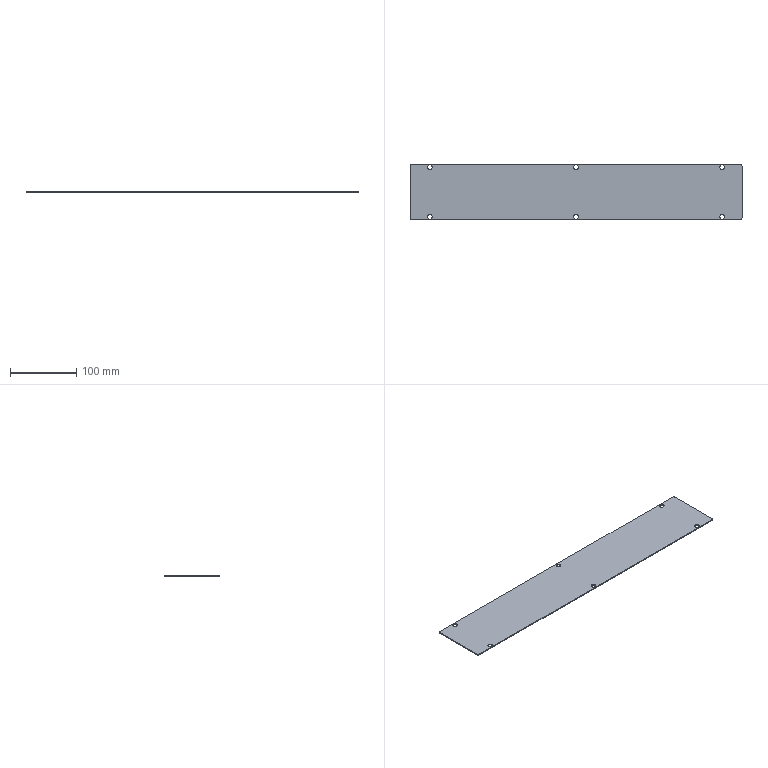Part | SolidWorks | features Cut 1, Extrusion 1, Fillet 1 | 1 solid | 22 faces | box 500 x 84 x 1.5 mm | volume 62642 mm3 | cylinder 16 | plane 6 | commonest cylinder face diameters 7 x12 6 x4
STEP:
#1=CARTESIAN_POINT('',(223.5,37.5,1.5));
#2=VERTEX_POINT('',#1);
#3=CARTESIAN_POINT('',(216.5,37.5,1.5));
#4=VERTEX_POINT('',#3);
#5=CARTESIAN_POINT('',(220.,37.5,1.5));
#6=DIRECTION('',(0.,0.,-1.));
#7=DIRECTION('',(1.,0.,0.));
#8=AXIS2_PLACEMENT_3D('',#5,#6,#7);
#9=CIRCLE('',#8,3.5);
#10=EDGE_CURVE('',#2,#4,#9,.T.);
#11=ORIENTED_EDGE('',*,*,#10,.F.);
#12=CARTESIAN_POINT('',(223.5,37.5,0.));
#13=VERTEX_POINT('',#12);
#14=CARTESIAN_POINT('',(223.5,37.5,1.5));
#15=DIRECTION('',(0.,0.,-1.));
#16=VECTOR('',#15,1000.);
#17=LINE('',#14,#16);
#18=EDGE_CURVE('',#2,#13,#17,.T.);
#19=ORIENTED_EDGE('',*,*,#18,.T.);
#20=CARTESIAN_POINT('',(216.5,37.5,0.));
#21=VERTEX_POINT('',#20);
#22=CARTESIAN_POINT('',(220.,37.5,0.));
#23=DIRECTION('',(0.,0.,-1.));
#24=DIRECTION('',(1.,0.,0.));
#25=AXIS2_PLACEMENT_3D('',#22,#23,#24);
#26=CIRCLE('',#25,3.5);
#27=EDGE_CURVE('',#13,#21,#26,.T.);
#28=ORIENTED_EDGE('',*,*,#27,.T.);
#29=CARTESIAN_POINT('',(216.5,37.5,1.5));
#30=DIRECTION('',(0.,0.,-1.));
#31=VECTOR('',#30,1000.);
#32=LINE('',#29,#31);
#33=EDGE_CURVE('',#4,#21,#32,.T.);
#34=ORIENTED_EDGE('',*,*,#33,.F.);
#35=EDGE_LOOP('',(#11,#19,#28,#34));
#36=FACE_OUTER_BOUND('',#35,.T.);
#37=CARTESIAN_POINT('',(220.,37.5,1.5));
#38=DIRECTION('',(0.,0.,-1.));
#39=DIRECTION('',(-1.,0.,0.));
#40=AXIS2_PLACEMENT_3D('',#37,#38,#39);
#41=CYLINDRICAL_SURFACE('',#40,3.5);
#42=ADVANCED_FACE('',(#36),#41,.F.);
#43=CARTESIAN_POINT('',(-216.5,37.5,1.5));
#44=VERTEX_POINT('',#43);
#45=CARTESIAN_POINT('',(-223.5,37.5,1.5));
#46=VERTEX_POINT('',#45);
#47=CARTESIAN_POINT('',(-220.,37.5,1.5));
#48=DIRECTION('',(0.,0.,-1.));
#49=DIRECTION('',(1.,0.,0.));
#50=AXIS2_PLACEMENT_3D('',#47,#48,#49);
#51=CIRCLE('',#50,3.5);
#52=EDGE_CURVE('',#44,#46,#51,.T.);
#53=ORIENTED_EDGE('',*,*,#52,.F.);
#54=CARTESIAN_POINT('',(-216.5,37.5,0.));
#55=VERTEX_POINT('',#54);
#56=CARTESIAN_POINT('',(-216.5,37.5,1.5));
#57=DIRECTION('',(0.,0.,-1.));
#58=VECTOR('',#57,1000.);
#59=LINE('',#56,#58);
#60=EDGE_CURVE('',#44,#55,#59,.T.);
#61=ORIENTED_EDGE('',*,*,#60,.T.);
#62=CARTESIAN_POINT('',(-223.5,37.5,0.));
#63=VERTEX_POINT('',#62);
#64=CARTESIAN_POINT('',(-220.,37.5,0.));
#65=DIRECTION('',(0.,0.,-1.));
#66=DIRECTION('',(1.,0.,0.));
#67=AXIS2_PLACEMENT_3D('',#64,#65,#66);
#68=CIRCLE('',#67,3.5);
#69=EDGE_CURVE('',#55,#63,#68,.T.);
#70=ORIENTED_EDGE('',*,*,#69,.T.);
#71=CARTESIAN_POINT('',(-223.5,37.5,1.5));
#72=DIRECTION('',(0.,0.,-1.));
#73=VECTOR('',#72,1000.);
#74=LINE('',#71,#73);
#75=EDGE_CURVE('',#46,#63,#74,.T.);
#76=ORIENTED_EDGE('',*,*,#75,.F.);
#77=EDGE_LOOP('',(#53,#61,#70,#76));
#78=FACE_OUTER_BOUND('',#77,.T.);
#79=CARTESIAN_POINT('',(-220.,37.5,1.5));
#80=DIRECTION('',(0.,0.,-1.));
#81=DIRECTION('',(-1.,0.,0.));
#82=AXIS2_PLACEMENT_3D('',#79,#80,#81);
#83=CYLINDRICAL_SURFACE('',#82,3.5);
#84=ADVANCED_FACE('',(#78),#83,.F.);
#85=CARTESIAN_POINT('',(3.5,-37.5,1.5));
#86=VERTEX_POINT('',#85);
#87=CARTESIAN_POINT('',(-3.5,-37.5,1.5));
#88=VERTEX_POINT('',#87);
#89=CARTESIAN_POINT('',(0.,-37.5,1.5));
#90=DIRECTION('',(0.,0.,-1.));
#91=DIRECTION('',(-1.,0.,0.));
#92=AXIS2_PLACEMENT_3D('',#89,#90,#91);
#93=CIRCLE('',#92,3.5);
#94=EDGE_CURVE('',#86,#88,#93,.T.);
#95=ORIENTED_EDGE('',*,*,#94,.F.);
#96=CARTESIAN_POINT('',(3.5,-37.5,0.));
#97=VERTEX_POINT('',#96);
#98=CARTESIAN_POINT('',(3.5,-37.5,1.5));
#99=DIRECTION('',(0.,0.,-1.));
#100=VECTOR('',#99,1000.);
#101=LINE('',#98,#100);
#102=EDGE_CURVE('',#86,#97,#101,.T.);
#103=ORIENTED_EDGE('',*,*,#102,.T.);
#104=CARTESIAN_POINT('',(-3.5,-37.5,0.));
#105=VERTEX_POINT('',#104);
#106=CARTESIAN_POINT('',(0.,-37.5,0.));
#107=DIRECTION('',(0.,0.,-1.));
#108=DIRECTION('',(-1.,0.,0.));
#109=AXIS2_PLACEMENT_3D('',#106,#107,#108);
#110=CIRCLE('',#109,3.5);
#111=EDGE_CURVE('',#97,#105,#110,.T.);
#112=ORIENTED_EDGE('',*,*,#111,.T.);
#113=CARTESIAN_POINT('',(-3.5,-37.5,1.5));
#114=DIRECTION('',(0.,0.,-1.));
#115=VECTOR('',#114,1000.);
#116=LINE('',#113,#115);
#117=EDGE_CURVE('',#88,#105,#116,.T.);
#118=ORIENTED_EDGE('',*,*,#117,.F.);
#119=EDGE_LOOP('',(#95,#103,#112,#118));
#120=FACE_OUTER_BOUND('',#119,.T.);
#121=CARTESIAN_POINT('',(0.,-37.5,1.5));
#122=DIRECTION('',(0.,0.,-1.));
#123=DIRECTION('',(-1.,0.,0.));
#124=AXIS2_PLACEMENT_3D('',#121,#122,#123);
#125=CYLINDRICAL_SURFACE('',#124,3.5);
#126=ADVANCED_FACE('',(#120),#125,.F.);
#127=CARTESIAN_POINT('',(-216.5,-37.5,1.5));
#128=VERTEX_POINT('',#127);
#129=CARTESIAN_POINT('',(-223.5,-37.5,1.5));
#130=VERTEX_POINT('',#129);
#131=CARTESIAN_POINT('',(-220.,-37.5,1.5));
#132=DIRECTION('',(0.,0.,-1.));
#133=DIRECTION('',(-1.,0.,0.));
#134=AXIS2_PLACEMENT_3D('',#131,#132,#133);
#135=CIRCLE('',#134,3.5);
#136=EDGE_CURVE('',#128,#130,#135,.T.);
#137=ORIENTED_EDGE('',*,*,#136,.F.);
#138=CARTESIAN_POINT('',(-216.5,-37.5,0.));
#139=VERTEX_POINT('',#138);
#140=CARTESIAN_POINT('',(-216.5,-37.5,1.5));
#141=DIRECTION('',(0.,0.,-1.));
#142=VECTOR('',#141,1000.);
#143=LINE('',#140,#142);
#144=EDGE_CURVE('',#128,#139,#143,.T.);
#145=ORIENTED_EDGE('',*,*,#144,.T.);
#146=CARTESIAN_POINT('',(-223.5,-37.5,0.));
#147=VERTEX_POINT('',#146);
#148=CARTESIAN_POINT('',(-220.,-37.5,0.));
#149=DIRECTION('',(0.,0.,-1.));
#150=DIRECTION('',(-1.,0.,0.));
#151=AXIS2_PLACEMENT_3D('',#148,#149,#150);
#152=CIRCLE('',#151,3.5);
#153=EDGE_CURVE('',#139,#147,#152,.T.);
#154=ORIENTED_EDGE('',*,*,#153,.T.);
#155=CARTESIAN_POINT('',(-223.5,-37.5,1.5));
#156=DIRECTION('',(0.,0.,-1.));
#157=VECTOR('',#156,1000.);
#158=LINE('',#155,#157);
#159=EDGE_CURVE('',#130,#147,#158,.T.);
#160=ORIENTED_EDGE('',*,*,#159,.F.);
#161=EDGE_LOOP('',(#137,#145,#154,#160));
#162=FACE_OUTER_BOUND('',#161,.T.);
#163=CARTESIAN_POINT('',(-220.,-37.5,1.5));
#164=DIRECTION('',(0.,0.,-1.));
#165=DIRECTION('',(-1.,0.,0.));
#166=AXIS2_PLACEMENT_3D('',#163,#164,#165);
#167=CYLINDRICAL_SURFACE('',#166,3.5);
#168=ADVANCED_FACE('',(#162),#167,.F.);
#169=CARTESIAN_POINT('',(223.5,-37.5,1.5));
#170=VERTEX_POINT('',#169);
#171=CARTESIAN_POINT('',(216.5,-37.5,1.5));
#172=VERTEX_POINT('',#171);
#173=CARTESIAN_POINT('',(220.,-37.5,1.5));
#174=DIRECTION('',(0.,0.,-1.));
#175=DIRECTION('',(-1.,0.,0.));
#176=AXIS2_PLACEMENT_3D('',#173,#174,#175);
#177=CIRCLE('',#176,3.5);
#178=EDGE_CURVE('',#170,#172,#177,.T.);
#179=ORIENTED_EDGE('',*,*,#178,.F.);
#180=CARTESIAN_POINT('',(223.5,-37.5,0.));
#181=VERTEX_POINT('',#180);
#182=CARTESIAN_POINT('',(223.5,-37.5,1.5));
#183=DIRECTION('',(0.,0.,-1.));
#184=VECTOR('',#183,1000.);
#185=LINE('',#182,#184);
#186=EDGE_CURVE('',#170,#181,#185,.T.);
#187=ORIENTED_EDGE('',*,*,#186,.T.);
#188=CARTESIAN_POINT('',(216.5,-37.5,0.));
#189=VERTEX_POINT('',#188);
#190=CARTESIAN_POINT('',(220.,-37.5,0.));
#191=DIRECTION('',(0.,0.,-1.));
#192=DIRECTION('',(-1.,0.,0.));
#193=AXIS2_PLACEMENT_3D('',#190,#191,#192);
#194=CIRCLE('',#193,3.5);
#195=EDGE_CURVE('',#181,#189,#194,.T.);
#196=ORIENTED_EDGE('',*,*,#195,.T.);
#197=CARTESIAN_POINT('',(216.5,-37.5,1.5));
#198=DIRECTION('',(0.,0.,-1.));
#199=VECTOR('',#198,1000.);
#200=LINE('',#197,#199);
#201=EDGE_CURVE('',#172,#189,#200,.T.);
#202=ORIENTED_EDGE('',*,*,#201,.F.);
#203=EDGE_LOOP('',(#179,#187,#196,#202));
#204=FACE_OUTER_BOUND('',#203,.T.);
#205=CARTESIAN_POINT('',(220.,-37.5,1.5));
#206=DIRECTION('',(0.,0.,-1.));
#207=DIRECTION('',(-1.,0.,0.));
#208=AXIS2_PLACEMENT_3D('',#205,#206,#207);
#209=CYLINDRICAL_SURFACE('',#208,3.5);
#210=ADVANCED_FACE('',(#204),#209,.F.);
#211=CARTESIAN_POINT('',(3.5,37.5,1.5));
#212=VERTEX_POINT('',#211);
#213=CARTESIAN_POINT('',(-3.5,37.5,1.5));
#214=VERTEX_POINT('',#213);
#215=CARTESIAN_POINT('',(0.,37.5,1.5));
#216=DIRECTION('',(0.,0.,-1.));
#217=DIRECTION('',(1.,0.,0.));
#218=AXIS2_PLACEMENT_3D('',#215,#216,#217);
#219=CIRCLE('',#218,3.5);
#220=EDGE_CURVE('',#212,#214,#219,.T.);
#221=ORIENTED_EDGE('',*,*,#220,.F.);
#222=CARTESIAN_POINT('',(3.5,37.5,0.));
#223=VERTEX_POINT('',#222);
#224=CARTESIAN_POINT('',(3.5,37.5,1.5));
#225=DIRECTION('',(0.,0.,-1.));
#226=VECTOR('',#225,1000.);
#227=LINE('',#224,#226);
#228=EDGE_CURVE('',#212,#223,#227,.T.);
#229=ORIENTED_EDGE('',*,*,#228,.T.);
#230=CARTESIAN_POINT('',(-3.5,37.5,0.));
#231=VERTEX_POINT('',#230);
#232=CARTESIAN_POINT('',(0.,37.5,0.));
#233=DIRECTION('',(0.,0.,-1.));
#234=DIRECTION('',(1.,0.,0.));
#235=AXIS2_PLACEMENT_3D('',#232,#233,#234);
#236=CIRCLE('',#235,3.5);
#237=EDGE_CURVE('',#223,#231,#236,.T.);
#238=ORIENTED_EDGE('',*,*,#237,.T.);
#239=CARTESIAN_POINT('',(-3.5,37.5,1.5));
#240=DIRECTION('',(0.,0.,-1.));
#241=VECTOR('',#240,1000.);
#242=LINE('',#239,#241);
#243=EDGE_CURVE('',#214,#231,#242,.T.);
#244=ORIENTED_EDGE('',*,*,#243,.F.);
#245=EDGE_LOOP('',(#221,#229,#238,#244));
#246=FACE_OUTER_BOUND('',#245,.T.);
#247=CARTESIAN_POINT('',(0.,37.5,1.5));
#248=DIRECTION('',(0.,0.,-1.));
#249=DIRECTION('',(-1.,0.,0.));
#250=AXIS2_PLACEMENT_3D('',#247,#248,#249);
#251=CYLINDRICAL_SURFACE('',#250,3.5);
#252=ADVANCED_FACE('',(#246),#251,.F.);
#253=CARTESIAN_POINT('',(250.,-39.,1.5));
#254=VERTEX_POINT('',#253);
#255=CARTESIAN_POINT('',(250.,39.,1.5));
#256=VERTEX_POINT('',#255);
#257=CARTESIAN_POINT('',(250.,42.,1.5));
#258=DIRECTION('',(0.,1.,0.));
#259=VECTOR('',#258,1000.);
#260=LINE('',#257,#259);
#261=EDGE_CURVE('',#254,#256,#260,.T.);
#262=ORIENTED_EDGE('',*,*,#261,.F.);
#263=CARTESIAN_POINT('',(250.,-39.,0.));
#264=VERTEX_POINT('',#263);
#265=CARTESIAN_POINT('',(250.,-39.,1.5));
#266=DIRECTION('',(0.,0.,-1.));
#267=VECTOR('',#266,1000.);
#268=LINE('',#265,#267);
#269=EDGE_CURVE('',#254,#264,#268,.T.);
#270=ORIENTED_EDGE('',*,*,#269,.T.);
#271=CARTESIAN_POINT('',(250.,39.,0.));
#272=VERTEX_POINT('',#271);
#273=CARTESIAN_POINT('',(250.,42.,0.));
#274=DIRECTION('',(0.,1.,0.));
#275=VECTOR('',#274,1000.);
#276=LINE('',#273,#275);
#277=EDGE_CURVE('',#264,#272,#276,.T.);
#278=ORIENTED_EDGE('',*,*,#277,.T.);
#279=CARTESIAN_POINT('',(250.,39.,1.5));
#280=DIRECTION('',(0.,0.,1.));
#281=VECTOR('',#280,1000.);
#282=LINE('',#279,#281);
#283=EDGE_CURVE('',#272,#256,#282,.T.);
#284=ORIENTED_EDGE('',*,*,#283,.T.);
#285=EDGE_LOOP('',(#262,#270,#278,#284));
#286=FACE_OUTER_BOUND('',#285,.T.);
#287=CARTESIAN_POINT('',(250.,42.,1.5));
#288=DIRECTION('',(-1.,0.,0.));
#289=DIRECTION('',(0.,0.,1.));
#290=AXIS2_PLACEMENT_3D('',#287,#288,#289);
#291=PLANE('',#290);
#292=ADVANCED_FACE('',(#286),#291,.F.);
#293=CARTESIAN_POINT('',(247.,42.,1.5));
#294=VERTEX_POINT('',#293);
#295=CARTESIAN_POINT('',(-247.,42.,1.5));
#296=VERTEX_POINT('',#295);
#297=CARTESIAN_POINT('',(-250.,42.,1.5));
#298=DIRECTION('',(-1.,0.,0.));
#299=VECTOR('',#298,1000.);
#300=LINE('',#297,#299);
#301=EDGE_CURVE('',#294,#296,#300,.T.);
#302=ORIENTED_EDGE('',*,*,#301,.F.);
#303=CARTESIAN_POINT('',(247.,42.,0.));
#304=VERTEX_POINT('',#303);
#305=CARTESIAN_POINT('',(247.,42.,1.5));
#306=DIRECTION('',(0.,0.,-1.));
#307=VECTOR('',#306,1000.);
#308=LINE('',#305,#307);
#309=EDGE_CURVE('',#294,#304,#308,.T.);
#310=ORIENTED_EDGE('',*,*,#309,.T.);
#311=CARTESIAN_POINT('',(-247.,42.,0.));
#312=VERTEX_POINT('',#311);
#313=CARTESIAN_POINT('',(-250.,42.,0.));
#314=DIRECTION('',(-1.,0.,0.));
#315=VECTOR('',#314,1000.);
#316=LINE('',#313,#315);
#317=EDGE_CURVE('',#304,#312,#316,.T.);
#318=ORIENTED_EDGE('',*,*,#317,.T.);
#319=CARTESIAN_POINT('',(-247.,42.,1.5));
#320=DIRECTION('',(0.,0.,1.));
#321=VECTOR('',#320,1000.);
#322=LINE('',#319,#321);
#323=EDGE_CURVE('',#312,#296,#322,.T.);
#324=ORIENTED_EDGE('',*,*,#323,.T.);
#325=EDGE_LOOP('',(#302,#310,#318,#324));
#326=FACE_OUTER_BOUND('',#325,.T.);
#327=CARTESIAN_POINT('',(-250.,42.,1.5));
#328=DIRECTION('',(0.,-1.,0.));
#329=DIRECTION('',(0.,0.,-1.));
#330=AXIS2_PLACEMENT_3D('',#327,#328,#329);
#331=PLANE('',#330);
#332=ADVANCED_FACE('',(#326),#331,.F.);
#333=CARTESIAN_POINT('',(-250.,39.,0.));
#334=VERTEX_POINT('',#333);
#335=CARTESIAN_POINT('',(-250.,-39.,0.));
#336=VERTEX_POINT('',#335);
#337=CARTESIAN_POINT('',(-250.,42.,0.));
#338=DIRECTION('',(0.,-1.,0.));
#339=VECTOR('',#338,1000.);
#340=LINE('',#337,#339);
#341=EDGE_CURVE('',#334,#336,#340,.T.);
#342=ORIENTED_EDGE('',*,*,#341,.T.);
#343=CARTESIAN_POINT('',(-250.,-39.,1.5));
#344=VERTEX_POINT('',#343);
#345=CARTESIAN_POINT('',(-250.,-39.,1.5));
#346=DIRECTION('',(0.,0.,1.));
#347=VECTOR('',#346,1000.);
#348=LINE('',#345,#347);
#349=EDGE_CURVE('',#336,#344,#348,.T.);
#350=ORIENTED_EDGE('',*,*,#349,.T.);
#351=CARTESIAN_POINT('',(-250.,39.,1.5));
#352=VERTEX_POINT('',#351);
#353=CARTESIAN_POINT('',(-250.,42.,1.5));
#354=DIRECTION('',(0.,-1.,0.));
#355=VECTOR('',#354,1000.);
#356=LINE('',#353,#355);
#357=EDGE_CURVE('',#352,#344,#356,.T.);
#358=ORIENTED_EDGE('',*,*,#357,.F.);
#359=CARTESIAN_POINT('',(-250.,39.,1.5));
#360=DIRECTION('',(0.,0.,-1.));
#361=VECTOR('',#360,1000.);
#362=LINE('',#359,#361);
#363=EDGE_CURVE('',#352,#334,#362,.T.);
#364=ORIENTED_EDGE('',*,*,#363,.T.);
#365=EDGE_LOOP('',(#342,#350,#358,#364));
#366=FACE_OUTER_BOUND('',#365,.T.);
#367=CARTESIAN_POINT('',(-250.,42.,1.5));
#368=DIRECTION('',(1.,0.,0.));
#369=DIRECTION('',(0.,0.,-1.));
#370=AXIS2_PLACEMENT_3D('',#367,#368,#369);
#371=PLANE('',#370);
#372=ADVANCED_FACE('',(#366),#371,.F.);
#373=CARTESIAN_POINT('',(-247.,-42.,0.));
#374=VERTEX_POINT('',#373);
#375=CARTESIAN_POINT('',(247.,-42.,0.));
#376=VERTEX_POINT('',#375);
#377=CARTESIAN_POINT('',(-250.,-42.,0.));
#378=DIRECTION('',(1.,0.,0.));
#379=VECTOR('',#378,1000.);
#380=LINE('',#377,#379);
#381=EDGE_CURVE('',#374,#376,#380,.T.);
#382=ORIENTED_EDGE('',*,*,#381,.T.);
#383=CARTESIAN_POINT('',(247.,-42.,1.5));
#384=VERTEX_POINT('',#383);
#385=CARTESIAN_POINT('',(247.,-42.,1.5));
#386=DIRECTION('',(0.,0.,1.));
#387=VECTOR('',#386,1000.);
#388=LINE('',#385,#387);
#389=EDGE_CURVE('',#376,#384,#388,.T.);
#390=ORIENTED_EDGE('',*,*,#389,.T.);
#391=CARTESIAN_POINT('',(-247.,-42.,1.5));
#392=VERTEX_POINT('',#391);
#393=CARTESIAN_POINT('',(-250.,-42.,1.5));
#394=DIRECTION('',(1.,0.,0.));
#395=VECTOR('',#394,1000.);
#396=LINE('',#393,#395);
#397=EDGE_CURVE('',#392,#384,#396,.T.);
#398=ORIENTED_EDGE('',*,*,#397,.F.);
#399=CARTESIAN_POINT('',(-247.,-42.,1.5));
#400=DIRECTION('',(0.,0.,-1.));
#401=VECTOR('',#400,1000.);
#402=LINE('',#399,#401);
#403=EDGE_CURVE('',#392,#374,#402,.T.);
#404=ORIENTED_EDGE('',*,*,#403,.T.);
#405=EDGE_LOOP('',(#382,#390,#398,#404));
#406=FACE_OUTER_BOUND('',#405,.T.);
#407=CARTESIAN_POINT('',(-250.,-42.,1.5));
#408=DIRECTION('',(0.,1.,0.));
#409=DIRECTION('',(0.,0.,1.));
#410=AXIS2_PLACEMENT_3D('',#407,#408,#409);
#411=PLANE('',#410);
#412=ADVANCED_FACE('',(#406),#411,.F.);
#413=CARTESIAN_POINT('',(220.,37.5,1.5));
#414=DIRECTION('',(0.,0.,-1.));
#415=DIRECTION('',(1.,0.,0.));
#416=AXIS2_PLACEMENT_3D('',#413,#414,#415);
#417=CIRCLE('',#416,3.5);
#418=EDGE_CURVE('',#4,#2,#417,.T.);
#419=ORIENTED_EDGE('',*,*,#418,.T.);
#420=ORIENTED_EDGE('',*,*,#10,.T.);
#421=EDGE_LOOP('',(#419,#420));
#422=FACE_BOUND('',#421,.T.);
#423=CARTESIAN_POINT('',(-220.,37.5,1.5));
#424=DIRECTION('',(0.,0.,-1.));
#425=DIRECTION('',(1.,0.,0.));
#426=AXIS2_PLACEMENT_3D('',#423,#424,#425);
#427=CIRCLE('',#426,3.5);
#428=EDGE_CURVE('',#46,#44,#427,.T.);
#429=ORIENTED_EDGE('',*,*,#428,.T.);
#430=ORIENTED_EDGE('',*,*,#52,.T.);
#431=EDGE_LOOP('',(#429,#430));
#432=FACE_BOUND('',#431,.T.);
#433=CARTESIAN_POINT('',(0.,-37.5,1.5));
#434=DIRECTION('',(0.,0.,-1.));
#435=DIRECTION('',(-1.,0.,0.));
#436=AXIS2_PLACEMENT_3D('',#433,#434,#435);
#437=CIRCLE('',#436,3.5);
#438=EDGE_CURVE('',#88,#86,#437,.T.);
#439=ORIENTED_EDGE('',*,*,#438,.T.);
#440=ORIENTED_EDGE('',*,*,#94,.T.);
#441=EDGE_LOOP('',(#439,#440));
#442=FACE_BOUND('',#441,.T.);
#443=CARTESIAN_POINT('',(-220.,-37.5,1.5));
#444=DIRECTION('',(0.,0.,-1.));
#445=DIRECTION('',(-1.,0.,0.));
#446=AXIS2_PLACEMENT_3D('',#443,#444,#445);
#447=CIRCLE('',#446,3.5);
#448=EDGE_CURVE('',#130,#128,#447,.T.);
#449=ORIENTED_EDGE('',*,*,#448,.T.);
#450=ORIENTED_EDGE('',*,*,#136,.T.);
#451=EDGE_LOOP('',(#449,#450));
#452=FACE_BOUND('',#451,.T.);
#453=CARTESIAN_POINT('',(220.,-37.5,1.5));
#454=DIRECTION('',(0.,0.,-1.));
#455=DIRECTION('',(-1.,0.,0.));
#456=AXIS2_PLACEMENT_3D('',#453,#454,#455);
#457=CIRCLE('',#456,3.5);
#458=EDGE_CURVE('',#172,#170,#457,.T.);
#459=ORIENTED_EDGE('',*,*,#458,.T.);
#460=ORIENTED_EDGE('',*,*,#178,.T.);
#461=EDGE_LOOP('',(#459,#460));
#462=FACE_BOUND('',#461,.T.);
#463=CARTESIAN_POINT('',(0.,37.5,1.5));
#464=DIRECTION('',(0.,0.,-1.));
#465=DIRECTION('',(1.,0.,0.));
#466=AXIS2_PLACEMENT_3D('',#463,#464,#465);
#467=CIRCLE('',#466,3.5);
#468=EDGE_CURVE('',#214,#212,#467,.T.);
#469=ORIENTED_EDGE('',*,*,#468,.T.);
#470=ORIENTED_EDGE('',*,*,#220,.T.);
#471=EDGE_LOOP('',(#469,#470));
#472=FACE_BOUND('',#471,.T.);
#473=ORIENTED_EDGE('',*,*,#397,.T.);
#474=CARTESIAN_POINT('',(247.,-39.,1.5));
#475=DIRECTION('',(0.,0.,1.));
#476=DIRECTION('',(1.,0.,0.));
#477=AXIS2_PLACEMENT_3D('',#474,#475,#476);
#478=CIRCLE('',#477,3.);
#479=EDGE_CURVE('',#384,#254,#478,.T.);
#480=ORIENTED_EDGE('',*,*,#479,.T.);
#481=ORIENTED_EDGE('',*,*,#261,.T.);
#482=CARTESIAN_POINT('',(247.,39.,1.5));
#483=DIRECTION('',(0.,0.,1.));
#484=DIRECTION('',(1.,0.,0.));
#485=AXIS2_PLACEMENT_3D('',#482,#483,#484);
#486=CIRCLE('',#485,3.);
#487=EDGE_CURVE('',#256,#294,#486,.T.);
#488=ORIENTED_EDGE('',*,*,#487,.T.);
#489=ORIENTED_EDGE('',*,*,#301,.T.);
#490=CARTESIAN_POINT('',(-247.,39.,1.5));
#491=DIRECTION('',(0.,0.,1.));
#492=DIRECTION('',(1.,0.,0.));
#493=AXIS2_PLACEMENT_3D('',#490,#491,#492);
#494=CIRCLE('',#493,3.);
#495=EDGE_CURVE('',#296,#352,#494,.T.);
#496=ORIENTED_EDGE('',*,*,#495,.T.);
#497=ORIENTED_EDGE('',*,*,#357,.T.);
#498=CARTESIAN_POINT('',(-247.,-39.,1.5));
#499=DIRECTION('',(0.,0.,1.));
#500=DIRECTION('',(1.,0.,0.));
#501=AXIS2_PLACEMENT_3D('',#498,#499,#500);
#502=CIRCLE('',#501,3.);
#503=EDGE_CURVE('',#344,#392,#502,.T.);
#504=ORIENTED_EDGE('',*,*,#503,.T.);
#505=EDGE_LOOP('',(#473,#480,#481,#488,#489,#496,#497,#504));
#506=FACE_OUTER_BOUND('',#505,.T.);
#507=CARTESIAN_POINT('',(0.,0.,1.5));
#508=DIRECTION('',(0.,0.,1.));
#509=DIRECTION('',(1.,0.,0.));
#510=AXIS2_PLACEMENT_3D('',#507,#508,#509);
#511=PLANE('',#510);
#512=ADVANCED_FACE('',(#422,#432,#442,#452,#462,#472,#506),#511,.T.);
#513=CARTESIAN_POINT('',(220.,37.5,0.));
#514=DIRECTION('',(0.,0.,-1.));
#515=DIRECTION('',(1.,0.,0.));
#516=AXIS2_PLACEMENT_3D('',#513,#514,#515);
#517=CIRCLE('',#516,3.5);
#518=EDGE_CURVE('',#21,#13,#517,.T.);
#519=ORIENTED_EDGE('',*,*,#518,.F.);
#520=ORIENTED_EDGE('',*,*,#27,.F.);
#521=EDGE_LOOP('',(#519,#520));
#522=FACE_BOUND('',#521,.T.);
#523=CARTESIAN_POINT('',(-220.,37.5,0.));
#524=DIRECTION('',(0.,0.,-1.));
#525=DIRECTION('',(1.,0.,0.));
#526=AXIS2_PLACEMENT_3D('',#523,#524,#525);
#527=CIRCLE('',#526,3.5);
#528=EDGE_CURVE('',#63,#55,#527,.T.);
#529=ORIENTED_EDGE('',*,*,#528,.F.);
#530=ORIENTED_EDGE('',*,*,#69,.F.);
#531=EDGE_LOOP('',(#529,#530));
#532=FACE_BOUND('',#531,.T.);
#533=CARTESIAN_POINT('',(0.,-37.5,0.));
#534=DIRECTION('',(0.,0.,-1.));
#535=DIRECTION('',(-1.,0.,0.));
#536=AXIS2_PLACEMENT_3D('',#533,#534,#535);
#537=CIRCLE('',#536,3.5);
#538=EDGE_CURVE('',#105,#97,#537,.T.);
#539=ORIENTED_EDGE('',*,*,#538,.F.);
#540=ORIENTED_EDGE('',*,*,#111,.F.);
#541=EDGE_LOOP('',(#539,#540));
#542=FACE_BOUND('',#541,.T.);
#543=CARTESIAN_POINT('',(-220.,-37.5,0.));
#544=DIRECTION('',(0.,0.,-1.));
#545=DIRECTION('',(-1.,0.,0.));
#546=AXIS2_PLACEMENT_3D('',#543,#544,#545);
#547=CIRCLE('',#546,3.5);
#548=EDGE_CURVE('',#147,#139,#547,.T.);
#549=ORIENTED_EDGE('',*,*,#548,.F.);
#550=ORIENTED_EDGE('',*,*,#153,.F.);
#551=EDGE_LOOP('',(#549,#550));
#552=FACE_BOUND('',#551,.T.);
#553=CARTESIAN_POINT('',(220.,-37.5,0.));
#554=DIRECTION('',(0.,0.,-1.));
#555=DIRECTION('',(-1.,0.,0.));
#556=AXIS2_PLACEMENT_3D('',#553,#554,#555);
#557=CIRCLE('',#556,3.5);
#558=EDGE_CURVE('',#189,#181,#557,.T.);
#559=ORIENTED_EDGE('',*,*,#558,.F.);
#560=ORIENTED_EDGE('',*,*,#195,.F.);
#561=EDGE_LOOP('',(#559,#560));
#562=FACE_BOUND('',#561,.T.);
#563=CARTESIAN_POINT('',(0.,37.5,0.));
#564=DIRECTION('',(0.,0.,-1.));
#565=DIRECTION('',(1.,0.,0.));
#566=AXIS2_PLACEMENT_3D('',#563,#564,#565);
#567=CIRCLE('',#566,3.5);
#568=EDGE_CURVE('',#231,#223,#567,.T.);
#569=ORIENTED_EDGE('',*,*,#568,.F.);
#570=ORIENTED_EDGE('',*,*,#237,.F.);
#571=EDGE_LOOP('',(#569,#570));
#572=FACE_BOUND('',#571,.T.);
#573=ORIENTED_EDGE('',*,*,#277,.F.);
#574=CARTESIAN_POINT('',(247.,-39.,0.));
#575=DIRECTION('',(0.,0.,-1.));
#576=DIRECTION('',(1.,0.,0.));
#577=AXIS2_PLACEMENT_3D('',#574,#575,#576);
#578=CIRCLE('',#577,3.);
#579=EDGE_CURVE('',#264,#376,#578,.T.);
#580=ORIENTED_EDGE('',*,*,#579,.T.);
#581=ORIENTED_EDGE('',*,*,#381,.F.);
#582=CARTESIAN_POINT('',(-247.,-39.,0.));
#583=DIRECTION('',(0.,0.,-1.));
#584=DIRECTION('',(1.,0.,0.));
#585=AXIS2_PLACEMENT_3D('',#582,#583,#584);
#586=CIRCLE('',#585,3.);
#587=EDGE_CURVE('',#374,#336,#586,.T.);
#588=ORIENTED_EDGE('',*,*,#587,.T.);
#589=ORIENTED_EDGE('',*,*,#341,.F.);
#590=CARTESIAN_POINT('',(-247.,39.,0.));
#591=DIRECTION('',(0.,0.,-1.));
#592=DIRECTION('',(1.,0.,0.));
#593=AXIS2_PLACEMENT_3D('',#590,#591,#592);
#594=CIRCLE('',#593,3.);
#595=EDGE_CURVE('',#334,#312,#594,.T.);
#596=ORIENTED_EDGE('',*,*,#595,.T.);
#597=ORIENTED_EDGE('',*,*,#317,.F.);
#598=CARTESIAN_POINT('',(247.,39.,0.));
#599=DIRECTION('',(0.,0.,-1.));
#600=DIRECTION('',(1.,0.,0.));
#601=AXIS2_PLACEMENT_3D('',#598,#599,#600);
#602=CIRCLE('',#601,3.);
#603=EDGE_CURVE('',#304,#272,#602,.T.);
#604=ORIENTED_EDGE('',*,*,#603,.T.);
#605=EDGE_LOOP('',(#573,#580,#581,#588,#589,#596,#597,#604));
#606=FACE_OUTER_BOUND('',#605,.T.);
#607=CARTESIAN_POINT('',(0.,0.,0.));
#608=DIRECTION('',(0.,0.,1.));
#609=DIRECTION('',(1.,0.,0.));
#610=AXIS2_PLACEMENT_3D('',#607,#608,#609);
#611=PLANE('',#610);
#612=ADVANCED_FACE('',(#522,#532,#542,#552,#562,#572,#606),#611,.F.);
#613=ORIENTED_EDGE('',*,*,#228,.F.);
#614=ORIENTED_EDGE('',*,*,#468,.F.);
#615=ORIENTED_EDGE('',*,*,#243,.T.);
#616=ORIENTED_EDGE('',*,*,#568,.T.);
#617=EDGE_LOOP('',(#613,#614,#615,#616));
#618=FACE_OUTER_BOUND('',#617,.T.);
#619=CARTESIAN_POINT('',(0.,37.5,1.5));
#620=DIRECTION('',(0.,0.,-1.));
#621=DIRECTION('',(-1.,0.,0.));
#622=AXIS2_PLACEMENT_3D('',#619,#620,#621);
#623=CYLINDRICAL_SURFACE('',#622,3.5);
#624=ADVANCED_FACE('',(#618),#623,.F.);
#625=ORIENTED_EDGE('',*,*,#186,.F.);
#626=ORIENTED_EDGE('',*,*,#458,.F.);
#627=ORIENTED_EDGE('',*,*,#201,.T.);
#628=ORIENTED_EDGE('',*,*,#558,.T.);
#629=EDGE_LOOP('',(#625,#626,#627,#628));
#630=FACE_OUTER_BOUND('',#629,.T.);
#631=CARTESIAN_POINT('',(220.,-37.5,1.5));
#632=DIRECTION('',(0.,0.,-1.));
#633=DIRECTION('',(-1.,0.,0.));
#634=AXIS2_PLACEMENT_3D('',#631,#632,#633);
#635=CYLINDRICAL_SURFACE('',#634,3.5);
#636=ADVANCED_FACE('',(#630),#635,.F.);
#637=ORIENTED_EDGE('',*,*,#144,.F.);
#638=ORIENTED_EDGE('',*,*,#448,.F.);
#639=ORIENTED_EDGE('',*,*,#159,.T.);
#640=ORIENTED_EDGE('',*,*,#548,.T.);
#641=EDGE_LOOP('',(#637,#638,#639,#640));
#642=FACE_OUTER_BOUND('',#641,.T.);
#643=CARTESIAN_POINT('',(-220.,-37.5,1.5));
#644=DIRECTION('',(0.,0.,-1.));
#645=DIRECTION('',(-1.,0.,0.));
#646=AXIS2_PLACEMENT_3D('',#643,#644,#645);
#647=CYLINDRICAL_SURFACE('',#646,3.5);
#648=ADVANCED_FACE('',(#642),#647,.F.);
#649=ORIENTED_EDGE('',*,*,#102,.F.);
#650=ORIENTED_EDGE('',*,*,#438,.F.);
#651=ORIENTED_EDGE('',*,*,#117,.T.);
#652=ORIENTED_EDGE('',*,*,#538,.T.);
#653=EDGE_LOOP('',(#649,#650,#651,#652));
#654=FACE_OUTER_BOUND('',#653,.T.);
#655=CARTESIAN_POINT('',(0.,-37.5,1.5));
#656=DIRECTION('',(0.,0.,-1.));
#657=DIRECTION('',(-1.,0.,0.));
#658=AXIS2_PLACEMENT_3D('',#655,#656,#657);
#659=CYLINDRICAL_SURFACE('',#658,3.5);
#660=ADVANCED_FACE('',(#654),#659,.F.);
#661=ORIENTED_EDGE('',*,*,#60,.F.);
#662=ORIENTED_EDGE('',*,*,#428,.F.);
#663=ORIENTED_EDGE('',*,*,#75,.T.);
#664=ORIENTED_EDGE('',*,*,#528,.T.);
#665=EDGE_LOOP('',(#661,#662,#663,#664));
#666=FACE_OUTER_BOUND('',#665,.T.);
#667=CARTESIAN_POINT('',(-220.,37.5,1.5));
#668=DIRECTION('',(0.,0.,-1.));
#669=DIRECTION('',(-1.,0.,0.));
#670=AXIS2_PLACEMENT_3D('',#667,#668,#669);
#671=CYLINDRICAL_SURFACE('',#670,3.5);
#672=ADVANCED_FACE('',(#666),#671,.F.);
#673=ORIENTED_EDGE('',*,*,#18,.F.);
#674=ORIENTED_EDGE('',*,*,#418,.F.);
#675=ORIENTED_EDGE('',*,*,#33,.T.);
#676=ORIENTED_EDGE('',*,*,#518,.T.);
#677=EDGE_LOOP('',(#673,#674,#675,#676));
#678=FACE_OUTER_BOUND('',#677,.T.);
#679=CARTESIAN_POINT('',(220.,37.5,1.5));
#680=DIRECTION('',(0.,0.,-1.));
#681=DIRECTION('',(-1.,0.,0.));
#682=AXIS2_PLACEMENT_3D('',#679,#680,#681);
#683=CYLINDRICAL_SURFACE('',#682,3.5);
#684=ADVANCED_FACE('',(#678),#683,.F.);
#685=ORIENTED_EDGE('',*,*,#479,.F.);
#686=ORIENTED_EDGE('',*,*,#389,.F.);
#687=ORIENTED_EDGE('',*,*,#579,.F.);
#688=ORIENTED_EDGE('',*,*,#269,.F.);
#689=EDGE_LOOP('',(#685,#686,#687,#688));
#690=FACE_OUTER_BOUND('',#689,.T.);
#691=CARTESIAN_POINT('',(247.,-39.,1.5));
#692=DIRECTION('',(0.,0.,-1.));
#693=DIRECTION('',(-1.,0.,0.));
#694=AXIS2_PLACEMENT_3D('',#691,#692,#693);
#695=CYLINDRICAL_SURFACE('',#694,3.);
#696=ADVANCED_FACE('',(#690),#695,.T.);
#697=ORIENTED_EDGE('',*,*,#487,.F.);
#698=ORIENTED_EDGE('',*,*,#283,.F.);
#699=ORIENTED_EDGE('',*,*,#603,.F.);
#700=ORIENTED_EDGE('',*,*,#309,.F.);
#701=EDGE_LOOP('',(#697,#698,#699,#700));
#702=FACE_OUTER_BOUND('',#701,.T.);
#703=CARTESIAN_POINT('',(247.,39.,1.5));
#704=DIRECTION('',(0.,0.,-1.));
#705=DIRECTION('',(-1.,0.,0.));
#706=AXIS2_PLACEMENT_3D('',#703,#704,#705);
#707=CYLINDRICAL_SURFACE('',#706,3.);
#708=ADVANCED_FACE('',(#702),#707,.T.);
#709=ORIENTED_EDGE('',*,*,#503,.F.);
#710=ORIENTED_EDGE('',*,*,#349,.F.);
#711=ORIENTED_EDGE('',*,*,#587,.F.);
#712=ORIENTED_EDGE('',*,*,#403,.F.);
#713=EDGE_LOOP('',(#709,#710,#711,#712));
#714=FACE_OUTER_BOUND('',#713,.T.);
#715=CARTESIAN_POINT('',(-247.,-39.,1.5));
#716=DIRECTION('',(0.,0.,-1.));
#717=DIRECTION('',(-1.,0.,0.));
#718=AXIS2_PLACEMENT_3D('',#715,#716,#717);
#719=CYLINDRICAL_SURFACE('',#718,3.);
#720=ADVANCED_FACE('',(#714),#719,.T.);
#721=ORIENTED_EDGE('',*,*,#495,.F.);
#722=ORIENTED_EDGE('',*,*,#323,.F.);
#723=ORIENTED_EDGE('',*,*,#595,.F.);
#724=ORIENTED_EDGE('',*,*,#363,.F.);
#725=EDGE_LOOP('',(#721,#722,#723,#724));
#726=FACE_OUTER_BOUND('',#725,.T.);
#727=CARTESIAN_POINT('',(-247.,39.,1.5));
#728=DIRECTION('',(0.,0.,-1.));
#729=DIRECTION('',(-1.,0.,0.));
#730=AXIS2_PLACEMENT_3D('',#727,#728,#729);
#731=CYLINDRICAL_SURFACE('',#730,3.);
#732=ADVANCED_FACE('',(#726),#731,.T.);
#733=CLOSED_SHELL('',(#42,#84,#126,#168,#210,#252,#292,#332,#372,#412,#512,#612,#624,#636,#648,#660,#672,#684,#696,#708,#720,#732));
#734=MANIFOLD_SOLID_BREP('',#733);
#735=CARTESIAN_POINT('',(0.,0.,0.));
#736=DIRECTION('',(0.,0.,1.));
#737=DIRECTION('',(1.,0.,0.));
#738=AXIS2_PLACEMENT_3D('',#735,#736,#737);
#739=(LENGTH_UNIT()NAMED_UNIT(*)SI_UNIT(.MILLI.,.METRE.));
#740=UNCERTAINTY_MEASURE_WITH_UNIT(LENGTH_MEASURE(0.00001),#739,'','');
#741=(NAMED_UNIT(*)PLANE_ANGLE_UNIT()SI_UNIT($,.RADIAN.));
#742=(NAMED_UNIT(*)SI_UNIT($,.STERADIAN.)SOLID_ANGLE_UNIT());
#743=(GEOMETRIC_REPRESENTATION_CONTEXT(3)GLOBAL_UNCERTAINTY_ASSIGNED_CONTEXT((#740))GLOBAL_UNIT_ASSIGNED_CONTEXT((#739,#741,#742))REPRESENTATION_CONTEXT('',''));
#744=ADVANCED_BREP_SHAPE_REPRESENTATION('',(#734,#738),#743);